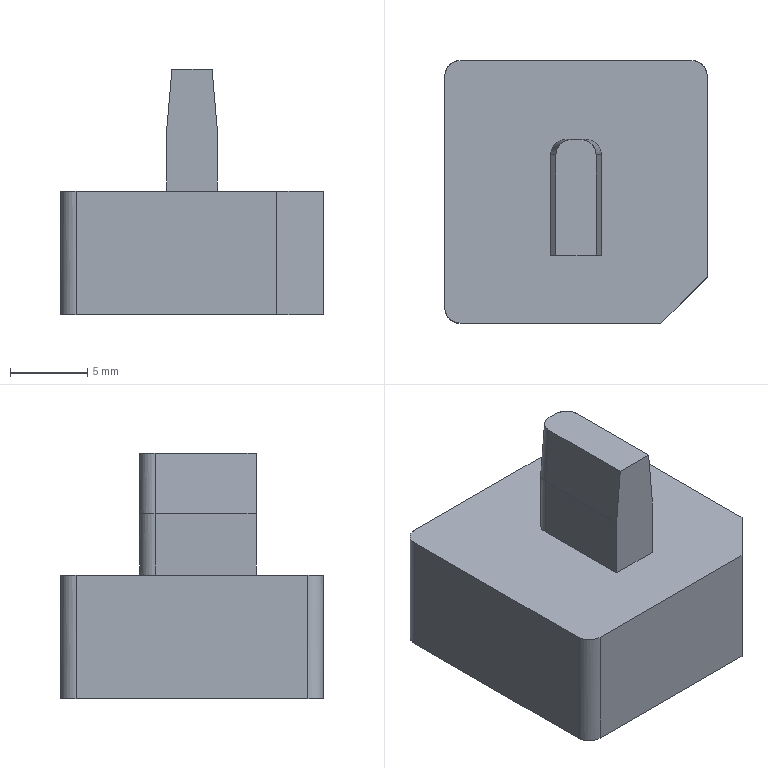NC program | PowerMill | posted with a generic post | part box 17 x 17 x 15.883 mm
Lines 3516 to 4335 of 37483:
N3613 M6
N3614 S18000 M03
N3615 G00 G90 X0.0 Y0.0
N3616 G43 Z10.804 H14
N3617
N3618 G05 P10000 R8
N3619 X2.2323 Y-6.6343
N3620 Z0.9272
N3621 G01 Z-0.2728 F1200.0
N3622 X2.2253 Y-6.5842 F2000.0
N3623 X2.2144 Y-6.5349
N3624 X2.1996 Y-6.4866
N3625 X2.1811 Y-6.4396
N3626 X2.1589 Y-6.3941
N3627 X2.1332 Y-6.3506
N3628 X2.1041 Y-6.3093
N3629 X2.0719 Y-6.2703
N3630 X2.0367 Y-6.2341
N3631 X1.9987 Y-6.2007
N3632 X1.9583 Y-6.1705
N3633 X1.9156 Y-6.1435
N3634 X1.8709 Y-6.12
N3635 X1.8244 Y-6.1
N3636 X1.7765 Y-6.0838
N3637 X1.7275 Y-6.0715
N3638 X1.6777 Y-6.063
N3639 X1.6274 Y-6.0585
N3640 X1.5769 Y-6.0579
N3641 X1.532 Y-6.0608
N3642 X1.4627 Y-6.0677
N3643 X1.3771 Y-6.0727
N3644 X1.2973 Y-6.0757
N3645 X1.2088 Y-6.0761
N3646 X1.0967 Y-6.0749
N3647 X0.616 Y-6.0742
N3648 X-0.0506 Y-6.0751
N3649 X-0.7111 Y-6.075
N3650 X-1.2122
N3651 X-1.2771 Y-6.0748
N3652 X-1.342 Y-6.0738
N3653 X-1.4069 Y-6.0715
N3654 X-1.4716 Y-6.0671
N3655 X-1.5361 Y-6.0602
N3656 X-1.6002 Y-6.0507
N3657 X-1.6641 Y-6.0393
N3658 X-1.7277 Y-6.0263
N3659 X-1.8102 Y-6.0058
N3660 X-1.8922 Y-5.9814
N3661 X-1.9734 Y-5.953
N3662 X-2.0536 Y-5.9208
N3663 X-2.1334 Y-5.8847
N3664 X-2.2103 Y-5.8456
N3665 X-2.2848 Y-5.8033
N3666 X-2.3594 Y-5.7564
N3667 X-2.4317 Y-5.7063
N3668 X-2.5016 Y-5.6529
N3669 X-2.5689 Y-5.5965
N3670 X-2.6335 Y-5.5372
N3671 X-2.6953 Y-5.4751
N3672 X-2.754 Y-5.4103
N3673 X-2.8097 Y-5.343
N3674 X-2.8623 Y-5.2732
N3675 X-2.9115 Y-5.2011
N3676 X-2.9575 Y-5.1269
N3677 X-3.0004 Y-5.05
N3678 X-3.0398 Y-4.9712
N3679 X-3.0755 Y-4.8906
N3680 X-3.1077 Y-4.8084
N3681 X-3.1361 Y-4.7247
N3682 X-3.1591 Y-4.646
N3683 X-3.1784 Y-4.5664
N3684 X-3.1941 Y-4.4859
N3685 X-3.2065 Y-4.4029
N3686 X-3.2156 Y-4.3153
N3687 X-3.2214 Y-4.2222
N3688 X-3.2238 Y-4.1226
N3689 Y-4.0172
N3690 X-3.2239 Y-2.0881
N3691 Y2.1886
N3692 Y2.3666
N3693 X-3.222 Y2.4807
N3694 X-3.2163 Y2.5913
N3695 X-3.207 Y2.6987
N3696 X-3.194 Y2.803
N3697 X-3.1773 Y2.9062
N3698 X-3.1562 Y3.0118
N3699 X-3.1311 Y3.1168
N3700 X-3.1022 Y3.2209
N3701 X-3.0694 Y3.324
N3702 X-3.0327 Y3.426
N3703 X-2.9922 Y3.5267
N3704 X-2.9481 Y3.626
N3705 X-2.9002 Y3.7238
N3706 X-2.8506 Y3.8163
N3707 X-2.7972 Y3.9076
N3708 X-2.7398 Y3.9978
N3709 X-2.6786 Y4.0865
N3710 X-2.6137 Y4.1734
N3711 X-2.5454 Y4.2584
N3712 X-2.4739 Y4.3409
N3713 X-2.3996 Y4.4206
N3714 X-2.3226 Y4.4973
N3715 X-2.2435 Y4.5706
N3716 X-2.1623 Y4.6404
N3717 X-2.079 Y4.7068
N3718 X-1.9924 Y4.7707
N3719 X-1.9033 Y4.8316
N3720 X-1.8117 Y4.8893
N3721 X-1.7179 Y4.9436
N3722 X-1.6222 Y4.9944
N3723 X-1.5247 Y5.0417
N3724 X-1.4258 Y5.0852
N3725 X-1.3255 Y5.125
N3726 X-1.2242 Y5.1609
N3727 X-1.1221 Y5.1928
N3728 X-1.0193 Y5.2209
N3729 X-0.9284 Y5.2424
N3730 X-0.8369 Y5.2615
N3731 X-0.7409 Y5.2783
N3732 X-0.6442 Y5.2916
N3733 X-0.5512 Y5.3008
N3734 X-0.458 Y5.3065
N3735 X-0.3647 Y5.3092
N3736 X-0.1411 Y5.3121
N3737 X0.1491 Y5.3126
N3738 X0.2886 Y5.3124
N3739 X0.3979 Y5.3104
N3740 X0.507 Y5.3043
N3741 X0.6156 Y5.2943
N3742 X0.7237 Y5.2803
N3743 X0.8309 Y5.2624
N3744 X0.9373 Y5.2406
N3745 X1.0426 Y5.215
N3746 X1.1468 Y5.1855
N3747 X1.2496 Y5.1523
N3748 X1.3511 Y5.1153
N3749 X1.4511 Y5.0746
N3750 X1.5496 Y5.0302
N3751 X1.6464 Y4.9822
N3752 X1.7413 Y4.9306
N3753 X1.8342 Y4.8756
N3754 X1.925 Y4.8172
N3755 X2.0139 Y4.7553
N3756 X2.1004 Y4.6901
N3757 X2.1844 Y4.6219
N3758 X2.2659 Y4.5505
N3759 X2.3447 Y4.4762
N3760 X2.4207 Y4.3991
N3761 X2.4937 Y4.3193
N3762 X2.5637 Y4.2368
N3763 X2.6306 Y4.1519
N3764 X2.6943 Y4.0646
N3765 X2.7547 Y3.975
N3766 X2.8117 Y3.8833
N3767 X2.865 Y3.79
N3768 X2.915 Y3.6945
N3769 X2.9615 Y3.597
N3770 X3.0045 Y3.4976
N3771 X3.0438 Y3.3966
N3772 X3.0793 Y3.2944
N3773 X3.111 Y3.1912
N3774 X3.1387 Y3.0871
N3775 X3.1624 Y2.9826
N3776 X3.1821 Y2.8784
N3777 X3.1979 Y2.773
N3778 X3.21 Y2.6654
N3779 X3.2184 Y2.5557
N3780 X3.223 Y2.4439
N3781 X3.2239 Y2.3299
N3782 Y-2.3577
N3783 X3.2236 Y-3.4462
N3784 X3.225 Y-4.0983
N3785 X3.2235 Y-4.1967
N3786 X3.2183 Y-4.2907
N3787 X3.2096 Y-4.3808
N3788 X3.1974 Y-4.4672
N3789 X3.1819 Y-4.5503
N3790 X3.1627 Y-4.6317
N3791 X3.1389 Y-4.716
N3792 X3.1112 Y-4.7991
N3793 X3.0797 Y-4.8809
N3794 X3.0445 Y-4.9613
N3795 X3.0056 Y-5.0402
N3796 X2.9632 Y-5.1172
N3797 X2.9175 Y-5.1919
N3798 X2.8684 Y-5.2645
N3799 X2.816 Y-5.3348
N3800 X2.7605 Y-5.4027
N3801 X2.702 Y-5.4679
N3802 X2.6405 Y-5.5305
N3803 X2.5762 Y-5.5901
N3804 X2.5093 Y-5.6468
N3805 X2.4399 Y-5.7003
N3806 X2.3682 Y-5.7507
N3807 X2.2942 Y-5.7977
N3808 X2.2182 Y-5.8412
N3809 X2.1405 Y-5.8813
N3810 X2.0612 Y-5.9176
N3811 X1.9804 Y-5.9503
N3812 X1.8982 Y-5.9793
N3813 X1.8144 Y-6.0045
N3814 X1.7293 Y-6.0261
N3815 X1.6426 Y-6.0439
N3816 X1.5546 Y-6.0579
N3817 X1.532 Y-6.0608
N3818 X1.4919 Y-6.064 Z-0.2729
N3819 X1.4518 Y-6.068
N3820 X1.4118 Y-6.0721 Z-0.273
N3821 X1.3716 Y-6.0742
N3822 X1.3314 Y-6.0748 Z-0.2731
N3823 X1.2912
N3824 X0.3479 Y-6.075 Z-0.2743
N3825 X-0.4589 Z-0.2754
N3826 X-1.13 Y-6.0745 Z-0.2762
N3827 X-1.3276 Y-6.0739 Z-0.2765
N3828 X-1.4114 Y-6.0715 Z-0.2766
N3829 X-1.4954 Y-6.0652 Z-0.2767
N3830 X-1.5798 Y-6.0549 Z-0.2768
N3831 X-1.6642 Y-6.0406 Z-0.2769
N3832 X-1.7487 Y-6.0222 Z-0.277
N3833 X-1.8329 Y-5.9998 Z-0.2771
N3834 X-1.9167 Y-5.9734 Z-0.2772
N3835 X-1.9998 Y-5.943 Z-0.2773
N3836 X-2.0807 Y-5.9093 Z-0.2774
N3837 X-2.16 Y-5.8718 Z-0.2775
N3838 X-2.2376 Y-5.8308 Z-0.2777
N3839 X-2.3132 Y-5.7864 Z-0.2778
N3840 X-2.3867 Y-5.7385 Z-0.2779
N3841 X-2.4579 Y-5.6873 Z-0.278
N3842 X-2.5268 Y-5.6329 Z-0.2781
N3843 X-2.5931 Y-5.5754 Z-0.2782
N3844 X-2.6567 Y-5.515 Z-0.2783
N3845 X-2.7174 Y-5.4518 Z-0.2784
N3846 X-2.7752 Y-5.3859 Z-0.2785
N3847 X-2.83 Y-5.3174 Z-0.2787
N3848 X-2.8816 Y-5.2465 Z-0.2788
N3849 X-2.9299 Y-5.1734 Z-0.2789
N3850 X-2.9747 Y-5.0982 Z-0.279
N3851 X-3.016 Y-5.0211 Z-0.2791
N3852 X-3.0537 Y-4.9423 Z-0.2792
N3853 X-3.0875 Y-4.8626 Z-0.2793
N3854 X-3.118 Y-4.7805 Z-0.2794
N3855 X-3.1452 Y-4.6957 Z-0.2795
N3856 X-3.1692 Y-4.6081 Z-0.2797
N3857 X-3.1864 Y-4.5328 Z-0.2798
N3858 X-3.2003 Y-4.4545 Z-0.2799
N3859 X-3.2112 Y-4.3715 Z-0.28
N3860 X-3.2188 Y-4.2826 Z-0.2801
N3861 X-3.2233 Y-4.1864 Z-0.2802
N3862 X-3.2245 Y-4.0983 Z-0.2803
N3863 X-3.2248 Y-1.646 Z-0.2834
N3864 X-3.2251 Y1.4077 Z-0.2873
N3865 X-3.2257 Y2.3666 Z-0.2885
N3866 X-3.2238 Y2.4778 Z-0.2886
N3867 X-3.218 Y2.5881 Z-0.2888
N3868 X-3.2083 Y2.6974 Z-0.2889
N3869 X-3.1947 Y2.8056 Z-0.2891
N3870 X-3.1772 Y2.9126 Z-0.2892
N3871 X-3.1559 Y3.0185 Z-0.2893
N3872 X-3.1308 Y3.1231 Z-0.2895
N3873 X-3.102 Y3.2264 Z-0.2896
N3874 X-3.0693 Y3.3283 Z-0.2897
N3875 X-3.033 Y3.4288 Z-0.2899
N3876 X-2.993 Y3.5279 Z-0.29
N3877 X-2.9482 Y3.6281 Z-0.2901
N3878 X-2.9002 Y3.7258 Z-0.2903
N3879 X-2.8491 Y3.8208 Z-0.2904
N3880 X-2.795 Y3.9131 Z-0.2906
N3881 X-2.7379 Y4.0026 Z-0.2907
N3882 X-2.6778 Y4.0896 Z-0.2908
N3883 X-2.6129 Y4.1767 Z-0.291
N3884 X-2.5451 Y4.261 Z-0.2911
N3885 X-2.4744 Y4.3426 Z-0.2912
N3886 X-2.4008 Y4.4214 Z-0.2914
N3887 X-2.3244 Y4.4974 Z-0.2915
N3888 X-2.2451 Y4.5707 Z-0.2916
N3889 X-2.163 Y4.6411 Z-0.2918
N3890 X-2.0782 Y4.7086 Z-0.2919
N3891 X-1.9905 Y4.7731 Z-0.2921
N3892 X-1.903 Y4.8329 Z-0.2922
N3893 X-1.8127 Y4.8897 Z-0.2923
N3894 X-1.7195 Y4.9436 Z-0.2925
N3895 X-1.6236 Y4.9945 Z-0.2926
N3896 X-1.5264 Y5.0416 Z-0.2927
N3897 X-1.4276 Y5.0851 Z-0.2929
N3898 X-1.3273 Y5.1249 Z-0.293
N3899 X-1.2257 Y5.161 Z-0.2931
N3900 X-1.1228 Y5.1932 Z-0.2933
N3901 X-1.0188 Y5.2216 Z-0.2934
N3902 X-0.9268 Y5.2433 Z-0.2935
N3903 X-0.8342 Y5.2621 Z-0.2937
N3904 X-0.7291 Y5.2798 Z-0.2938
N3905 X-0.6327 Y5.2928 Z-0.2939
N3906 X-0.5386 Y5.302 Z-0.294
N3907 X-0.4443 Y5.3081 Z-0.2942
N3908 X-0.3371 Y5.3118 Z-0.2943
N3909 X-0.234 Y5.3121 Z-0.2944
N3910 X0.2886 Y5.3122 Z-0.2951
N3911 X0.3978 Y5.3103 Z-0.2952
N3912 X0.5066 Y5.3044 Z-0.2954
N3913 X0.6151 Y5.2946 Z-0.2955
N3914 X0.7232 Y5.2807 Z-0.2956
N3915 X0.8301 Y5.2631 Z-0.2958
N3916 X0.9361 Y5.2415 Z-0.2959
N3917 X1.0412 Y5.216 Z-0.296
N3918 X1.1451 Y5.1867 Z-0.2962
N3919 X1.2478 Y5.1536 Z-0.2963
N3920 X1.3479 Y5.1172 Z-0.2965
N3921 X1.4475 Y5.0768 Z-0.2966
N3922 X1.5467 Y5.0323 Z-0.2967
N3923 X1.6443 Y4.9841 Z-0.2969
N3924 X1.7396 Y4.9326 Z-0.297
N3925 X1.8318 Y4.8784 Z-0.2971
N3926 X1.921 Y4.8213 Z-0.2973
N3927 X2.01 Y4.7596 Z-0.2974
N3928 X2.0968 Y4.6947 Z-0.2975
N3929 X2.181 Y4.6266 Z-0.2977
N3930 X2.2627 Y4.5555 Z-0.2978
N3931 X2.3417 Y4.4814 Z-0.298
N3932 X2.4178 Y4.4045 Z-0.2981
N3933 X2.491 Y4.3249 Z-0.2982
N3934 X2.5612 Y4.2427 Z-0.2984
N3935 X2.6282 Y4.158 Z-0.2985
N3936 X2.6921 Y4.0708 Z-0.2986
N3937 X2.7527 Y3.9815 Z-0.2988
N3938 X2.8099 Y3.8899 Z-0.2989
N3939 X2.8637 Y3.7965 Z-0.2991
N3940 X2.9139 Y3.7011 Z-0.2992
N3941 X2.9607 Y3.6038 Z-0.2993
N3942 X3.0039 Y3.5047 Z-0.2995
N3943 X3.0435 Y3.4038 Z-0.2996
N3944 X3.0795 Y3.301 Z-0.2997
N3945 X3.1108 Y3.2001 Z-0.2999
N3946 X3.1384 Y3.0976 Z-0.3
N3947 X3.1623 Y2.9934 Z-0.3001
N3948 X3.1825 Y2.8877 Z-0.3003
N3949 X3.1989 Y2.7803 Z-0.3004
N3950 X3.2116 Y2.6716 Z-0.3006
N3951 X3.2204 Y2.5615 Z-0.3007
N3952 X3.2252 Y2.4502 Z-0.3008
N3953 X3.2263 Y2.3378 Z-0.301
N3954 X3.2267 Y-0.7455 Z-0.3049
N3955 X3.227 Y-2.3578 Z-0.3069
N3956 X3.2277 Y-3.8881 Z-0.3089
N3957 X3.228 Y-4.0983 Z-0.3091
N3958 X3.2264 Y-4.1946 Z-0.3092
N3959 X3.2213 Y-4.288 Z-0.3094
N3960 X3.2126 Y-4.3785 Z-0.3095
N3961 X3.2004 Y-4.4663 Z-0.3096
N3962 X3.1845 Y-4.5516 Z-0.3097
N3963 X3.1652 Y-4.6348 Z-0.3098
N3964 X3.1423 Y-4.7158 Z-0.3099
N3965 X3.116 Y-4.7952 Z-0.31
N3966 X3.0845 Y-4.8774 Z-0.3101
N3967 X3.0493 Y-4.958 Z-0.3102
N3968 X3.0106 Y-5.0369 Z-0.3104
N3969 X2.9682 Y-5.114 Z-0.3105
N3970 X2.9225 Y-5.1891 Z-0.3106
N3971 X2.8734 Y-5.2619 Z-0.3107
N3972 X2.821 Y-5.3325 Z-0.3108
N3973 X2.7656 Y-5.4004 Z-0.3109
N3974 X2.7073 Y-5.4657 Z-0.311
N3975 X2.646 Y-5.5283 Z-0.3111
N3976 X2.582 Y-5.588 Z-0.3112
N3977 X2.5152 Y-5.6447 Z-0.3114
N3978 X2.446 Y-5.6984 Z-0.3115
N3979 X2.3744 Y-5.7488 Z-0.3116
N3980 X2.3005 Y-5.796 Z-0.3117
N3981 X2.2244 Y-5.8398 Z-0.3118
N3982 X2.1465 Y-5.88 Z-0.3119
N3983 X2.0669 Y-5.9167 Z-0.312
N3984 X1.9857 Y-5.9496 Z-0.3121
N3985 X1.9031 Y-5.9789 Z-0.3122
N3986 X1.8193 Y-6.0043 Z-0.3123
N3987 X1.7344 Y-6.0259 Z-0.3125
N3988 X1.6486 Y-6.0436 Z-0.3126
N3989 X1.5621 Y-6.0573 Z-0.3127
N3990 X1.5321 Y-6.0612
N3991 X1.4542 Y-6.0696 Z-0.3128
N3992 X1.3759 Y-6.0741 Z-0.3129
N3993 X1.2976 Y-6.0748 Z-0.313
N3994 X-0.6932 Y-6.0745 Z-0.3155
N3995 X-1.3276 Y-6.0741 Z-0.3163
N3996 X-1.4104 Y-6.072 Z-0.3164
N3997 X-1.4936 Y-6.066 Z-0.3165
N3998 X-1.5774 Y-6.0559 Z-0.3167
N3999 X-1.6615 Y-6.0418 Z-0.3168
N4000 X-1.7459 Y-6.0236 Z-0.3169
N4001 X-1.8304 Y-6.0014 Z-0.317
N4002 X-1.9148 Y-5.975 Z-0.3171
N4003 X-1.9989 Y-5.9445 Z-0.3172
N4004 X-2.0794 Y-5.9113 Z-0.3173
N4005 X-2.1584 Y-5.8744 Z-0.3174
N4006 X-2.2358 Y-5.8339 Z-0.3175
N4007 X-2.3112 Y-5.7898 Z-0.3176
N4008 X-2.3847 Y-5.7423 Z-0.3178
N4009 X-2.4561 Y-5.6914 Z-0.3179
N4010 X-2.5251 Y-5.6372 Z-0.318
N4011 X-2.5916 Y-5.5799 Z-0.3181
N4012 X-2.6554 Y-5.5197 Z-0.3182
N4013 X-2.7165 Y-5.4566 Z-0.3183
N4014 X-2.7745 Y-5.3909 Z-0.3184
N4015 X-2.8295 Y-5.3226 Z-0.3185
N4016 X-2.8814 Y-5.2518 Z-0.3186
N4017 X-2.9299 Y-5.1789 Z-0.3188
N4018 X-2.9749 Y-5.1039 Z-0.3189
N4019 X-3.0165 Y-5.027 Z-0.319
N4020 X-3.0545 Y-4.9482 Z-0.3191
N4021 X-3.0889 Y-4.8679 Z-0.3192
N4022 X-3.1197 Y-4.7856 Z-0.3193
N4023 X-3.1472 Y-4.7012 Z-0.3194
N4024 X-3.1711 Y-4.6146 Z-0.3195
N4025 X-3.1892 Y-4.5356 Z-0.3196
N4026 X-3.2036 Y-4.4558 Z-0.3197
N4027 X-3.2144 Y-4.375 Z-0.3198
N4028 X-3.2221 Y-4.2883 Z-0.32
N4029 X-3.2267 Y-4.1941 Z-0.3201
N4030 X-3.228 Y-4.0983 Z-0.3202
N4031 X-3.2283 Y-1.4004 Z-0.3236
N4032 X-3.2287 Y1.799 Z-0.3277
N4033 X-3.2288 Y2.3666 Z-0.3284
N4034 X-3.2271 Y2.4743 Z-0.3285
N4035 X-3.2219 Y2.5813 Z-0.3286
N4036 X-3.2129 Y2.6875 Z-0.3288
N4037 X-3.2002 Y2.7932 Z-0.3289
N4038 X-3.1836 Y2.8982 Z-0.3291
N4039 X-3.1631 Y3.0028 Z-0.3292
N4040 X-3.1386 Y3.1069 Z-0.3293
N4041 X-3.1102 Y3.2107 Z-0.3295
N4042 X-3.0777 Y3.314 Z-0.3296
N4043 X-3.0428 Y3.4127 Z-0.3297
N4044 X-3.0041 Y3.5107 Z-0.3299
N4045 X-2.9613 Y3.6082 Z-0.33
N4046 X-2.9145 Y3.705 Z-0.3301
N4047 X-2.8635 Y3.8012 Z-0.3303
N4048 X-2.8097 Y3.8945 Z-0.3304
N4049 X-2.7526 Y3.9857 Z-0.3305
N4050 X-2.6921 Y4.0748 Z-0.3307
N4051 X-2.6283 Y4.1615 Z-0.3308
N4052 X-2.5614 Y4.2459 Z-0.331
N4053 X-2.4912 Y4.3278 Z-0.3311
N4054 X-2.418 Y4.4073 Z-0.3312
N4055 X-2.3417 Y4.4841 Z-0.3314
N4056 X-2.2624 Y4.5583 Z-0.3315
N4057 X-2.1812 Y4.6288 Z-0.3316
N4058 X-2.0974 Y4.6965 Z-0.3318
N4059 X-2.011 Y4.761 Z-0.3319
N4060 X-1.9222 Y4.8225 Z-0.332
N4061 X-1.831 Y4.8806 Z-0.3322
N4062 X-1.7375 Y4.9355 Z-0.3323
N4063 X-1.642 Y4.987 Z-0.3325
N4064 X-1.5456 Y5.0344 Z-0.3326
N4065 X-1.4475 Y5.0783 Z-0.3327
N4066 X-1.3476 Y5.1186 Z-0.3329
N4067 X-1.246 Y5.1553 Z-0.333
N4068 X-1.1429 Y5.1883 Z-0.3331
N4069 X-1.0384 Y5.2175 Z-0.3333
N4070 X-0.9327 Y5.243 Z-0.3334
N4071 X-0.8259 Y5.2645 Z-0.3336
N4072 X-0.7235 Y5.2814 Z-0.3337
N4073 X-0.62 Y5.2946 Z-0.3338
N4074 X-0.5137 Y5.3041 Z-0.3339
N4075 X-0.4044 Y5.31 Z-0.3341
N4076 X-0.2918 Y5.312 Z-0.3342
N4077 X-0.1759 Y5.3121 Z-0.3344
N4078 X0.2886 Y5.3123 Z-0.335
N4079 X0.3981 Y5.3104 Z-0.3351
N4080 X0.5073 Y5.3045 Z-0.3352
N4081 X0.616 Y5.2947 Z-0.3354
N4082 X0.7241 Y5.2809 Z-0.3355
N4083 X0.8314 Y5.2632 Z-0.3357
N4084 X0.9378 Y5.2416 Z-0.3358
N4085 X1.0431 Y5.2162 Z-0.3359
N4086 X1.1474 Y5.1869 Z-0.3361
N4087 X1.2503 Y5.1538 Z-0.3362
N4088 X1.3518 Y5.117 Z-0.3363
N4089 X1.4519 Y5.0765 Z-0.3365
N4090 X1.5503 Y5.0324 Z-0.3366
N4091 X1.647 Y4.9846 Z-0.3367
N4092 X1.7418 Y4.9334 Z-0.3369
N4093 X1.8347 Y4.8786 Z-0.337
N4094 X1.9257 Y4.8204 Z-0.3372
N4095 X2.0148 Y4.7587 Z-0.3373
N4096 X2.1014 Y4.6938 Z-0.3374
N4097 X2.1855 Y4.6258 Z-0.3376
N4098 X2.267 Y4.5548 Z-0.3377
N4099 X2.3457 Y4.4809 Z-0.3378
N4100 X2.4217 Y4.4042 Z-0.338
N4101 X2.4947 Y4.3247 Z-0.3381
N4102 X2.5647 Y4.2426 Z-0.3383
N4103 X2.6317 Y4.1578 Z-0.3384
N4104 X2.6956 Y4.0706 Z-0.3385
N4105 X2.7562 Y3.9811 Z-0.3387
N4106 X2.8136 Y3.8893 Z-0.3388
N4107 X2.8677 Y3.7952 Z-0.3389
N4108 X2.9181 Y3.6994 Z-0.3391
N4109 X2.965 Y3.6019 Z-0.3392
N4110 X3.0082 Y3.5028 Z-0.3393
N4111 X3.0476 Y3.4024 Z-0.3395
N4112 X3.0832 Y3.3007 Z-0.3396
N4113 X3.115 Y3.1979 Z-0.3398
N4114 X3.1429 Y3.0942 Z-0.3399
N4115 X3.1669 Y2.9895 Z-0.34
N4116 X3.187 Y2.884 Z-0.3402
N4117 X3.2033 Y2.7774 Z-0.3403
N4118 X3.2158 Y2.6691 Z-0.3404
N4119 X3.2244 Y2.5594 Z-0.3406
N4120 X3.2292 Y2.4484 Z-0.3407
N4121 X3.2302 Y2.3362 Z-0.3409
N4122 X3.23 Y-0.0769 Z-0.3439
N4123 X3.2305 Y-2.3578 Z-0.3468
N4124 X3.2312 Y-3.8966 Z-0.3487
N4125 X3.2315 Y-4.0983 Z-0.349
N4126 X3.2299 Y-4.1946 Z-0.3491
N4127 X3.2248 Y-4.288 Z-0.3492
N4128 X3.2161 Y-4.3784 Z-0.3494
N4129 X3.2038 Y-4.4663 Z-0.3495
N4130 X3.188 Y-4.5517 Z-0.3496
N4131 X3.1686 Y-4.6348 Z-0.3497
N4132 X3.1458 Y-4.7159 Z-0.3498
N4133 X3.1194 Y-4.7953 Z-0.3499
N4134 X3.088 Y-4.8774 Z-0.35
N4135 X3.0528 Y-4.958 Z-0.3501
N4136 X3.014 Y-5.0369 Z-0.3502
N4137 X2.9717 Y-5.114 Z-0.3503
N4138 X2.9259 Y-5.1891 Z-0.3505
N4139 X2.8768 Y-5.262 Z-0.3506
N4140 X2.8244 Y-5.3326 Z-0.3507
N4141 X2.7692 Y-5.4003 Z-0.3508
N4142 X2.711 Y-5.4655 Z-0.3509
N4143 X2.6499 Y-5.5279 Z-0.351
N4144 X2.586 Y-5.5875 Z-0.3511
N4145 X2.5194 Y-5.6442 Z-0.3512
N4146 X2.4502 Y-5.6978 Z-0.3513
N4147 X2.3786 Y-5.7483 Z-0.3515
N4148 X2.3047 Y-5.7955 Z-0.3516
N4149 X2.2287 Y-5.8393 Z-0.3517
N4150 X2.1507 Y-5.8797 Z-0.3518
N4151 X2.0711 Y-5.9164 Z-0.3519
N4152 X1.9899 Y-5.9494 Z-0.352
N4153 X1.9074 Y-5.9786 Z-0.3521
N4154 X1.8238 Y-6.004 Z-0.3522
N4155 X1.7391 Y-6.0256 Z-0.3523
N4156 X1.6536 Y-6.0433 Z-0.3524
N4157 X1.5673 Y-6.057 Z-0.3526
N4158 X1.5321 Y-6.0615
N4159 X1.4533 Y-6.0698 Z-0.3527
N4160 X1.3742 Y-6.0742 Z-0.3528
N4161 X1.295 Y-6.0749 Z-0.3529
N4162 X0.1207 Z-0.3544
N4163 X-0.8474 Y-6.075 Z-0.3556
N4164 X-1.3276 Y-6.074 Z-0.3562
N4165 X-1.4129 Y-6.0717 Z-0.3563
N4166 X-1.4981 Y-6.0654 Z-0.3564
N4167 X-1.5834 Y-6.0551 Z-0.3565
N4168 X-1.6686 Y-6.0408 Z-0.3567
N4169 X-1.7535 Y-6.0225 Z-0.3568
N4170 X-1.8378 Y-6.0003 Z-0.3569
N4171 X-1.9216 Y-5.974 Z-0.357
N4172 X-2.0045 Y-5.9439 Z-0.3571
N4173 X-2.0854 Y-5.9103 Z-0.3572
N4174 X-2.1648 Y-5.873 Z-0.3573
N4175 X-2.2424 Y-5.8321 Z-0.3574
N4176 X-2.318 Y-5.7877 Z-0.3575
N4177 X-2.3916 Y-5.7399 Z-0.3577
N4178 X-2.4629 Y-5.6888 Z-0.3578
N4179 X-2.5318 Y-5.6345 Z-0.3579
N4180 X-2.5982 Y-5.5771 Z-0.358
N4181 X-2.6619 Y-5.5168 Z-0.3581
N4182 X-2.7227 Y-5.4537 Z-0.3582
N4183 X-2.7806 Y-5.3878 Z-0.3583
N4184 X-2.8355 Y-5.3194 Z-0.3584
N4185 X-2.8871 Y-5.2486 Z-0.3585
N4186 X-2.9355 Y-5.1755 Z-0.3586
N4187 X-2.9804 Y-5.1004 Z-0.3588
N4188 X-3.0218 Y-5.0234 Z-0.3589
N4189 X-3.0597 Y-4.9446 Z-0.359
N4190 X-3.0938 Y-4.8643 Z-0.3591
N4191 X-3.1246 Y-4.7818 Z-0.3592
N4192 X-3.1519 Y-4.6971 Z-0.3593
N4193 X-3.1756 Y-4.6108 Z-0.3594
N4194 X-3.1935 Y-4.5316 Z-0.3595
N4195 X-3.2077 Y-4.4517 Z-0.3596
N4196 X-3.2184 Y-4.3698 Z-0.3597
N4197 X-3.2259 Y-4.2822 Z-0.3598
N4198 X-3.2303 Y-4.1872 Z-0.36
N4199 X-3.2315 Y-4.0983 Z-0.3601
N4200 X-3.2318 Y-1.5006 Z-0.3634
N4201 X-3.2322 Y1.656 Z-0.3674
N4202 X-3.2323 Y2.3666 Z-0.3683
N4203 X-3.2306 Y2.4745 Z-0.3684
N4204 X-3.2253 Y2.5817 Z-0.3685
N4205 X-3.2164 Y2.688 Z-0.3687
N4206 X-3.2036 Y2.7937 Z-0.3688
N4207 X-3.187 Y2.8989 Z-0.3689
N4208 X-3.1665 Y3.0034 Z-0.3691
N4209 X-3.142 Y3.1075 Z-0.3692
N4210 X-3.1135 Y3.2112 Z-0.3693
N4211 X-3.0811 Y3.3144 Z-0.3695
N4212 X-3.0461 Y3.4133 Z-0.3696
N4213 X-3.0073 Y3.5114 Z-0.3697
N4214 X-2.9645 Y3.6089 Z-0.3699
N4215 X-2.9176 Y3.7058 Z-0.37
N4216 X-2.8667 Y3.802 Z-0.3702
N4217 X-2.8137 Y3.894 Z-0.3703
N4218 X-2.7572 Y3.9842 Z-0.3704
N4219 X-2.6969 Y4.0728 Z-0.3706
N4220 X-2.6331 Y4.1596 Z-0.3707
N4221 X-2.5659 Y4.2443 Z-0.3708
N4222 X-2.4954 Y4.3268 Z-0.371
N4223 X-2.4217 Y4.4068 Z-0.3711
N4224 X-2.3451 Y4.484 Z-0.3712
N4225 X-2.2658 Y4.5583 Z-0.3714
N4226 X-2.1841 Y4.6294 Z-0.3715
N4227 X-2.1002 Y4.6971 Z-0.3717
N4228 X-2.0143 Y4.7614 Z-0.3718
N4229 X-1.9264 Y4.8222 Z-0.3719
N4230 X-1.8358 Y4.8799 Z-0.3721
N4231 X-1.7426 Y4.9347 Z-0.3722
N4232 X-1.6471 Y4.9861 Z-0.3723
N4233 X-1.5496 Y5.0341 Z-0.3725
N4234 X-1.4505 Y5.0784 Z-0.3726
N4235 X-1.3503 Y5.1189 Z-0.3727
N4236 X-1.249 Y5.1555 Z-0.3729
N4237 X-1.1472 Y5.1881 Z-0.373
N4238 X-1.0451 Y5.2166 Z-0.3731
N4239 X-0.9475 Y5.2401 Z-0.3733
N4240 X-0.8492 Y5.2606 Z-0.3734
N4241 X-0.7503 Y5.2778 Z-0.3735
N4242 X-0.6508 Y5.2916 Z-0.3737
N4243 X-0.5488 Y5.3018 Z-0.3738
N4244 X-0.4486 Y5.3083 Z-0.3739
N4245 X-0.3482 Y5.3115 Z-0.374
N4246 X-0.2479 Y5.312 Z-0.3742
N4247 X0.2886 Y5.3123 Z-0.3748
N4248 X0.399 Y5.3105 Z-0.375
N4249 X0.5088 Y5.3046 Z-0.3751
N4250 X0.6179 Y5.2948 Z-0.3753
N4251 X0.7262 Y5.2812 Z-0.3754
N4252 X0.8336 Y5.2636 Z-0.3755
N4253 X0.9399 Y5.2421 Z-0.3757
N4254 X1.0451 Y5.2168 Z-0.3758
N4255 X1.149 Y5.1877 Z-0.3759
N4256 X1.2515 Y5.1549 Z-0.3761
N4257 X1.3525 Y5.1184 Z-0.3762
N4258 X1.4521 Y5.0781 Z-0.3764
N4259 X1.5502 Y5.0342 Z-0.3765
N4260 X1.6426 Y4.9887 Z-0.3766
N4261 X1.7332 Y4.9399 Z-0.3768
N4262 X1.8278 Y4.8846 Z-0.3769
N4263 X1.9149 Y4.8296 Z-0.377
N4264 X2.0 Y4.7716 Z-0.3772
N4265 X2.0872 Y4.7074 Z-0.3773
N4266 X2.1717 Y4.6402 Z-0.3774
N4267 X2.2534 Y4.5701 Z-0.3776
N4268 X2.3322 Y4.4974 Z-0.3777
N4269 X2.4081 Y4.4218 Z-0.3778
N4270 X2.4823 Y4.3424 Z-0.378
N4271 X2.5533 Y4.2605 Z-0.3781
N4272 X2.6212 Y4.1761 Z-0.3782
N4273 X2.6859 Y4.0894 Z-0.3784
N4274 X2.7472 Y4.0005 Z-0.3785
N4275 X2.805 Y3.9096 Z-0.3787
N4276 X2.8594 Y3.8167 Z-0.3788
N4277 X2.9102 Y3.722 Z-0.3789
N4278 X2.9581 Y3.6244 Z-0.3791
N4279 X3.0021 Y3.5258 Z-0.3792
N4280 X3.0422 Y3.4262 Z-0.3793
N4281 X3.0785 Y3.3253 Z-0.3795
N4282 X3.1111 Y3.2229 Z-0.3796
N4283 X3.1399 Y3.1194 Z-0.3797
N4284 X3.1649 Y3.0145 Z-0.3799
N4285 X3.1861 Y2.9085 Z-0.38
N4286 X3.2034 Y2.8014 Z-0.3802
N4287 X3.2169 Y2.6932 Z-0.3803
N4288 X3.2265 Y2.5841 Z-0.3804
N4289 X3.2321 Y2.4741 Z-0.3806
N4290 X3.2338 Y2.3666 Z-0.3807
N4291 X3.2333 Y1.3481 Z-0.382
N4292 X3.2336 Y-0.3472 Z-0.3841
N4293 X3.234 Y-2.3578 Z-0.3867
N4294 X3.2348 Y-3.9934 Z-0.3887
N4295 X3.235 Y-4.0983 Z-0.3889
N4296 X3.2334 Y-4.1947 Z-0.389
N4297 X3.2282 Y-4.2881 Z-0.3891
N4298 X3.2195 Y-4.3787 Z-0.3892
N4299 X3.2073 Y-4.4665 Z-0.3893
N4300 X3.1914 Y-4.5519 Z-0.3895
N4301 X3.1721 Y-4.635 Z-0.3896
N4302 X3.1492 Y-4.7161 Z-0.3897
N4303 X3.1228 Y-4.7955 Z-0.3898
N4304 X3.0914 Y-4.8776 Z-0.3899
N4305 X3.0562 Y-4.9582 Z-0.39
N4306 X3.0174 Y-5.0371 Z-0.3901
N4307 X2.9751 Y-5.1142 Z-0.3902
N4308 X2.9293 Y-5.1893 Z-0.3903
N4309 X2.8802 Y-5.2622 Z-0.3904
N4310 X2.8278 Y-5.3328 Z-0.3906
N4311 X2.7727 Y-5.4004 Z-0.3907
N4312 X2.7146 Y-5.4654 Z-0.3908
N4313 X2.6536 Y-5.5278 Z-0.3909
N4314 X2.5897 Y-5.5874 Z-0.391
N4315 X2.5231 Y-5.644 Z-0.3911
N4316 X2.4539 Y-5.6977 Z-0.3912
N4317 X2.3822 Y-5.7482 Z-0.3913
N4318 X2.3083 Y-5.7954 Z-0.3914
N4319 X2.2323 Y-5.8393 Z-0.3916
N4320 X2.1543 Y-5.8796 Z-0.3917
N4321 X2.0747 Y-5.9163 Z-0.3918
N4322 X1.9935 Y-5.9493 Z-0.3919
N4323 X1.911 Y-5.9786 Z-0.392
N4324 X1.8274 Y-6.004 Z-0.3921
N4325 X1.7429 Y-6.0255 Z-0.3922
N4326 X1.6576 Y-6.0432 Z-0.3923
N4327 X1.5716 Y-6.0569 Z-0.3924
N4328 X1.5321 Y-6.0618 Z-0.3925
N4329 X1.4525 Y-6.07 Z-0.3926
N4330 X1.3725 Y-6.0743 Z-0.3927
N4331 X1.2924 Y-6.0749 Z-0.3928
N4332 X-0.3973 Y-6.075 Z-0.3949
N4333 X-1.3275 Y-6.0744 Z-0.3961
N4334 X-1.4116 Y-6.0723 Z-0.3962
N4335 X-1.4961 Y-6.0662 Z-0.3963
N4336 X-1.5809 Y-6.0561 Z-0.3964
N4337 X-1.666 Y-6.042 Z-0.3965
N4338 X-1.751 Y-6.0238 Z-0.3966
N4339 X-1.8359 Y-6.0016 Z-0.3968
N4340 X-1.9203 Y-5.9754 Z-0.3969
N4341 X-2.0041 Y-5.9452 Z-0.397
N4342 X-2.0847 Y-5.9121 Z-0.3971
N4343 X-2.1637 Y-5.8753 Z-0.3972
N4344 X-2.241 Y-5.8348 Z-0.3973
N4345 X-2.3166 Y-5.7908 Z-0.3974
N4346 X-2.3901 Y-5.7434 Z-0.3975
N4347 X-2.4615 Y-5.6925 Z-0.3976
N4348 X-2.5306 Y-5.6385 Z-0.3978
N4349 X-2.5971 Y-5.5813 Z-0.3979
N4350 X-2.661 Y-5.5211 Z-0.398
N4351 X-2.7221 Y-5.4581 Z-0.3981
N4352 X-2.7802 Y-5.3924 Z-0.3982
N4353 X-2.8353 Y-5.3241 Z-0.3983
N4354 X-2.8872 Y-5.2535 Z-0.3984
N4355 X-2.9358 Y-5.1806 Z-0.3985
N4356 X-2.9809 Y-5.1056 Z-0.3986
N4357 X-3.0226 Y-5.0287 Z-0.3987
N4358 X-3.0606 Y-4.9502 Z-0.3989
N4359 X-3.095 Y-4.8701 Z-0.399
N4360 X-3.126 Y-4.7877 Z-0.3991
N4361 X-3.1536 Y-4.703 Z-0.3992
N4362 X-3.1756 Y-4.6245 Z-0.3993
N4363 X-3.1942 Y-4.5454 Z-0.3994
N4364 X-3.2089 Y-4.4656 Z-0.3995
N4365 X-3.2202 Y-4.3839 Z-0.3996
N4366 X-3.2284 Y-4.2969 Z-0.3997
N4367 X-3.2333 Y-4.203 Z-0.3998
N4368 X-3.235 Y-4.1011 Z-0.4
N4369 Y-3.9929 Z-0.4001
N4370 X-3.2353 Y-1.293 Z-0.4035
N4371 X-3.2357 Y1.7532 Z-0.4074
N4372 X-3.2361 Y2.3666 Z-0.4081
N4373 X-3.2342 Y2.4782 Z-0.4083
N4374 X-3.2284 Y2.5885 Z-0.4084
N4375 X-3.2188 Y2.6976 Z-0.4086
N4376 X-3.2053 Y2.8055 Z-0.4087
N4377 X-3.1879 Y2.9123 Z-0.4088
N4378 X-3.1667 Y3.018 Z-0.409
N4379 X-3.1417 Y3.1228 Z-0.4091
N4380 X-3.1142 Y3.2217 Z-0.4092
N4381 X-3.0831 Y3.3195 Z-0.4094
N4382 X-3.0475 Y3.4186 Z-0.4095
N4383 X-3.0074 Y3.5185 Z-0.4096
N4384 X-2.9631 Y3.6183 Z-0.4098
N4385 X-2.915 Y3.717 Z-0.4099
N4386 X-2.8637 Y3.8129 Z-0.41
N4387 X-2.8101 Y3.9053 Z-0.4102
N4388 X-2.7544 Y3.9934 Z-0.4103
N4389 X-2.6965 Y4.0781 Z-0.4104
N4390 X-2.6318 Y4.1656 Z-0.4106
N4391 X-2.564 Y4.2506 Z-0.4107
N4392 X-2.4932 Y4.333 Z-0.4109
N4393 X-2.4194 Y4.4127 Z-0.411
N4394 X-2.3429 Y4.4895 Z-0.4111
N4395 X-2.2636 Y4.5634 Z-0.4113
N4396 X-2.1818 Y4.6342 Z-0.4114
N4397 X-2.0975 Y4.7019 Z-0.4115
N4398 X-2.0108 Y4.7664 Z-0.4117
N4399 X-1.9246 Y4.8257 Z-0.4118
N4400 X-1.8356 Y4.8822 Z-0.4119
N4401 X-1.7429 Y4.9363 Z-0.4121
N4402 X-1.6467 Y4.9879 Z-0.4122
N4403 X-1.5484 Y5.0362 Z-0.4124
N4404 X-1.4501 Y5.0802 Z-0.4125
N4405 X-1.352 Y5.1198 Z-0.4126
N4406 X-1.254 Y5.1552 Z-0.4128
N4407 X-1.1563 Y5.1863 Z-0.4129
N4408 X-1.0583 Y5.2134 Z-0.413
N4409 X-0.9464 Y5.2408 Z-0.4132
N4410 X-0.841 Y5.2628 Z-0.4133
N4411 X-0.7408 Y5.28 Z-0.4134
N4412 X-0.6449 Y5.2927 Z-0.4135
N4413 X-0.5492 Y5.3018 Z-0.4137
N4414 X-0.4375 Y5.3088 Z-0.4138
N4415 X-0.3237 Y5.3119 Z-0.414
N4416 X-0.2091 Y5.3121 Z-0.4141
N4417 X0.2886 Y5.3122 Z-0.4147
N4418 X0.4014 Y5.3103 Z-0.4149
N4419 X0.5124 Y5.3045 Z-0.415
N4420 X0.6215 Y5.2948 Z-0.4151
N4421 X0.7287 Y5.2814 Z-0.4153
N4422 X0.8341 Y5.2643 Z-0.4154
N4423 X0.9386 Y5.2433 Z-0.4156
N4424 X1.0436 Y5.2182 Z-0.4157
N4425 X1.1476 Y5.1892 Z-0.4158
N4426 X1.2506 Y5.1563 Z-0.416
N4427 X1.3524 Y5.1196 Z-0.4161
N4428 X1.4529 Y5.0791 Z-0.4162
N4429 X1.5518 Y5.035 Z-0.4164
N4430 X1.6487 Y4.9874 Z-0.4165
N4431 X1.7439 Y4.9362 Z-0.4166
N4432 X1.8372 Y4.8814 Z-0.4168